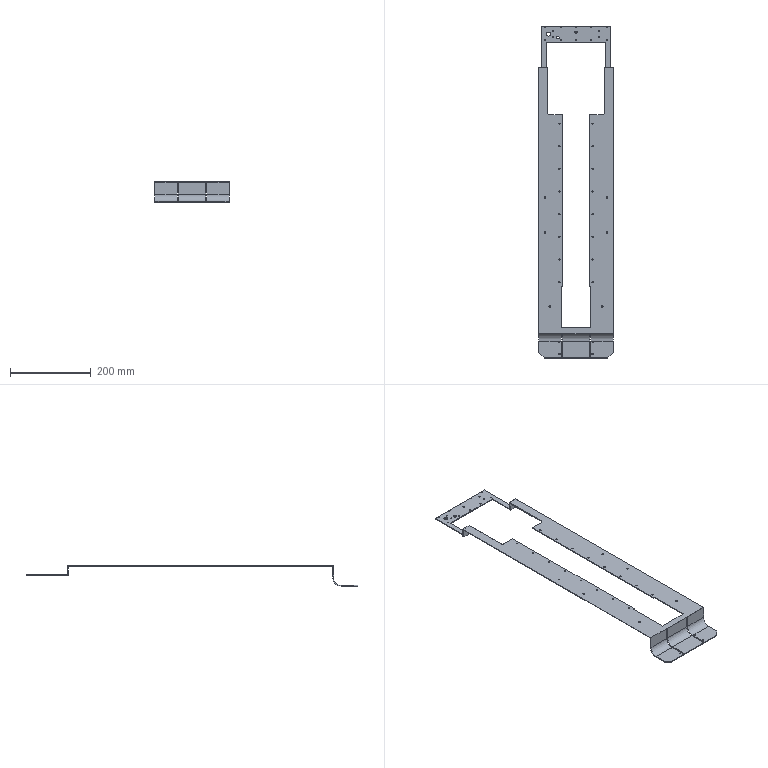Part | STEP file | 1-28.1 | 1 solid | 95 faces | box 184 x 821 x 50 mm | volume 191096 mm3 | cylinder 53 | plane 42 | commonest cylinder face diameters 3 x34 10 x5 4 x4 5 x3 36 x3 40 x3